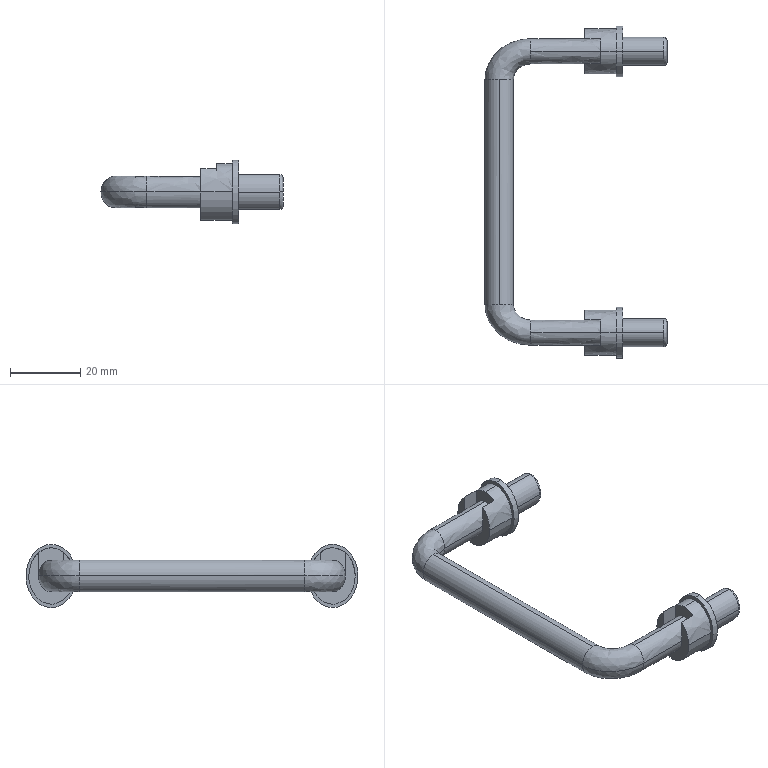Part | NX | features BREP 1 | 1 solid | 54 faces | box 51.75 x 94.4 x 18 mm | volume 11603 mm3 | spline 40 | plane 14